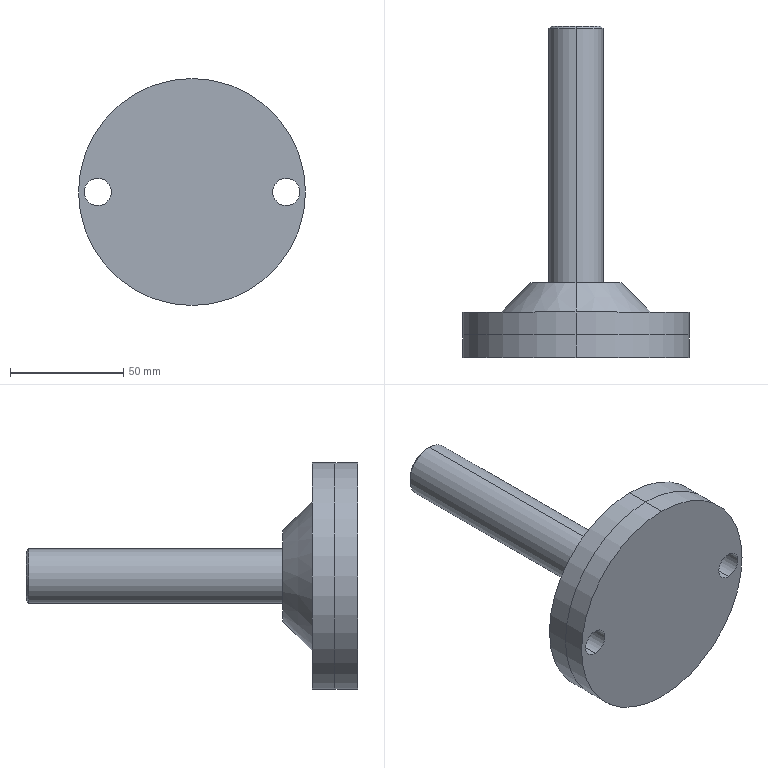Part | SolidWorks | features BaseBody 3 | 3 solids | 41 faces | box 100 x 146 x 100 mm | volume 232661 mm3 | cylinder 18 | plane 15 | cone 8 | commonest cylinder face diameters 12 x8 100 x4 24 x2 26 x2 30 x2
STEP:
#1=CARTESIAN_POINT('',(-41.5,-15.,-6.));
#2=VERTEX_POINT('',#1);
#3=CARTESIAN_POINT('',(-41.5,-15.,6.));
#4=VERTEX_POINT('',#3);
#5=CARTESIAN_POINT('',(-41.5,-15.,0.));
#6=DIRECTION('',(0.,1.,0.));
#7=DIRECTION('',(0.,0.,1.));
#8=AXIS2_PLACEMENT_3D('',#5,#6,#7);
#9=CIRCLE('',#8,6.);
#10=EDGE_CURVE('',#2,#4,#9,.T.);
#11=ORIENTED_EDGE('',*,*,#10,.F.);
#12=CARTESIAN_POINT('',(-41.5,-5.,-6.));
#13=VERTEX_POINT('',#12);
#14=CARTESIAN_POINT('',(-41.5,-15.,-6.));
#15=DIRECTION('',(0.,1.,0.));
#16=VECTOR('',#15,1000.);
#17=LINE('',#14,#16);
#18=EDGE_CURVE('',#2,#13,#17,.T.);
#19=ORIENTED_EDGE('',*,*,#18,.T.);
#20=CARTESIAN_POINT('',(-41.5,-5.,6.));
#21=VERTEX_POINT('',#20);
#22=CARTESIAN_POINT('',(-41.5,-5.,0.));
#23=DIRECTION('',(0.,1.,0.));
#24=DIRECTION('',(0.,0.,1.));
#25=AXIS2_PLACEMENT_3D('',#22,#23,#24);
#26=CIRCLE('',#25,6.);
#27=EDGE_CURVE('',#13,#21,#26,.T.);
#28=ORIENTED_EDGE('',*,*,#27,.T.);
#29=CARTESIAN_POINT('',(-41.5,-15.,6.));
#30=DIRECTION('',(0.,1.,0.));
#31=VECTOR('',#30,1000.);
#32=LINE('',#29,#31);
#33=EDGE_CURVE('',#4,#21,#32,.T.);
#34=ORIENTED_EDGE('',*,*,#33,.F.);
#35=EDGE_LOOP('',(#11,#19,#28,#34));
#36=FACE_OUTER_BOUND('',#35,.T.);
#37=CARTESIAN_POINT('',(-41.5,-15.,0.));
#38=DIRECTION('',(0.,1.,0.));
#39=DIRECTION('',(0.,0.,1.));
#40=AXIS2_PLACEMENT_3D('',#37,#38,#39);
#41=CYLINDRICAL_SURFACE('',#40,6.);
#42=ADVANCED_FACE('',(#36),#41,.F.);
#43=CARTESIAN_POINT('',(41.5,-15.,-6.));
#44=VERTEX_POINT('',#43);
#45=CARTESIAN_POINT('',(41.5,-15.,6.));
#46=VERTEX_POINT('',#45);
#47=CARTESIAN_POINT('',(41.5,-15.,0.));
#48=DIRECTION('',(0.,1.,0.));
#49=DIRECTION('',(0.,0.,1.));
#50=AXIS2_PLACEMENT_3D('',#47,#48,#49);
#51=CIRCLE('',#50,6.);
#52=EDGE_CURVE('',#44,#46,#51,.T.);
#53=ORIENTED_EDGE('',*,*,#52,.F.);
#54=CARTESIAN_POINT('',(41.5,-5.,-6.));
#55=VERTEX_POINT('',#54);
#56=CARTESIAN_POINT('',(41.5,-15.,-6.));
#57=DIRECTION('',(0.,1.,0.));
#58=VECTOR('',#57,1000.);
#59=LINE('',#56,#58);
#60=EDGE_CURVE('',#44,#55,#59,.T.);
#61=ORIENTED_EDGE('',*,*,#60,.T.);
#62=CARTESIAN_POINT('',(41.5,-5.,6.));
#63=VERTEX_POINT('',#62);
#64=CARTESIAN_POINT('',(41.5,-5.,0.));
#65=DIRECTION('',(0.,1.,0.));
#66=DIRECTION('',(0.,0.,1.));
#67=AXIS2_PLACEMENT_3D('',#64,#65,#66);
#68=CIRCLE('',#67,6.);
#69=EDGE_CURVE('',#55,#63,#68,.T.);
#70=ORIENTED_EDGE('',*,*,#69,.T.);
#71=CARTESIAN_POINT('',(41.5,-15.,6.));
#72=DIRECTION('',(0.,1.,0.));
#73=VECTOR('',#72,1000.);
#74=LINE('',#71,#73);
#75=EDGE_CURVE('',#46,#63,#74,.T.);
#76=ORIENTED_EDGE('',*,*,#75,.F.);
#77=EDGE_LOOP('',(#53,#61,#70,#76));
#78=FACE_OUTER_BOUND('',#77,.T.);
#79=CARTESIAN_POINT('',(41.5,-15.,0.));
#80=DIRECTION('',(0.,1.,0.));
#81=DIRECTION('',(0.,0.,1.));
#82=AXIS2_PLACEMENT_3D('',#79,#80,#81);
#83=CYLINDRICAL_SURFACE('',#82,6.);
#84=ADVANCED_FACE('',(#78),#83,.F.);
#85=CARTESIAN_POINT('',(0.,0.,13.));
#86=VERTEX_POINT('',#85);
#87=CARTESIAN_POINT('',(0.,0.,-13.));
#88=VERTEX_POINT('',#87);
#89=CARTESIAN_POINT('',(0.,0.,0.));
#90=DIRECTION('',(0.,-1.,0.));
#91=DIRECTION('',(0.,0.,-1.));
#92=AXIS2_PLACEMENT_3D('',#89,#90,#91);
#93=CIRCLE('',#92,13.);
#94=EDGE_CURVE('',#86,#88,#93,.T.);
#95=ORIENTED_EDGE('',*,*,#94,.T.);
#96=CARTESIAN_POINT('',(0.,8.,-13.));
#97=VERTEX_POINT('',#96);
#98=CARTESIAN_POINT('',(0.,8.,-13.));
#99=DIRECTION('',(0.,1.,0.));
#100=VECTOR('',#99,1000.);
#101=LINE('',#98,#100);
#102=EDGE_CURVE('',#88,#97,#101,.T.);
#103=ORIENTED_EDGE('',*,*,#102,.T.);
#104=CARTESIAN_POINT('',(0.,8.,13.));
#105=VERTEX_POINT('',#104);
#106=CARTESIAN_POINT('',(0.,8.,0.));
#107=DIRECTION('',(0.,1.,0.));
#108=DIRECTION('',(0.,0.,1.));
#109=AXIS2_PLACEMENT_3D('',#106,#107,#108);
#110=CIRCLE('',#109,13.);
#111=EDGE_CURVE('',#97,#105,#110,.T.);
#112=ORIENTED_EDGE('',*,*,#111,.T.);
#113=CARTESIAN_POINT('',(0.,8.,13.));
#114=DIRECTION('',(0.,1.,0.));
#115=VECTOR('',#114,1000.);
#116=LINE('',#113,#115);
#117=EDGE_CURVE('',#86,#105,#116,.T.);
#118=ORIENTED_EDGE('',*,*,#117,.F.);
#119=EDGE_LOOP('',(#95,#103,#112,#118));
#120=FACE_OUTER_BOUND('',#119,.T.);
#121=CARTESIAN_POINT('',(0.,8.,0.));
#122=DIRECTION('',(0.,1.,0.));
#123=DIRECTION('',(0.,0.,1.));
#124=AXIS2_PLACEMENT_3D('',#121,#122,#123);
#125=CYLINDRICAL_SURFACE('',#124,13.);
#126=ADVANCED_FACE('',(#120),#125,.F.);
#127=CARTESIAN_POINT('',(0.,8.,-20.));
#128=VERTEX_POINT('',#127);
#129=CARTESIAN_POINT('',(0.,8.,20.));
#130=VERTEX_POINT('',#129);
#131=CARTESIAN_POINT('',(0.,8.,0.));
#132=DIRECTION('',(0.,-1.,0.));
#133=DIRECTION('',(0.,0.,-1.));
#134=AXIS2_PLACEMENT_3D('',#131,#132,#133);
#135=CIRCLE('',#134,20.);
#136=EDGE_CURVE('',#128,#130,#135,.T.);
#137=ORIENTED_EDGE('',*,*,#136,.T.);
#138=CARTESIAN_POINT('',(0.,-5.,33.));
#139=VERTEX_POINT('',#138);
#140=CARTESIAN_POINT('',(0.,-5.,33.));
#141=DIRECTION('',(0.,-0.7071,0.7071));
#142=VECTOR('',#141,1000.);
#143=LINE('',#140,#142);
#144=EDGE_CURVE('',#130,#139,#143,.T.);
#145=ORIENTED_EDGE('',*,*,#144,.T.);
#146=CARTESIAN_POINT('',(0.,-5.,-33.));
#147=VERTEX_POINT('',#146);
#148=CARTESIAN_POINT('',(0.,-5.,0.));
#149=DIRECTION('',(0.,-1.,0.));
#150=DIRECTION('',(0.,0.,-1.));
#151=AXIS2_PLACEMENT_3D('',#148,#149,#150);
#152=CIRCLE('',#151,33.);
#153=EDGE_CURVE('',#147,#139,#152,.T.);
#154=ORIENTED_EDGE('',*,*,#153,.F.);
#155=CARTESIAN_POINT('',(0.,-5.,-33.));
#156=DIRECTION('',(0.,-0.7071,-0.7071));
#157=VECTOR('',#156,1000.);
#158=LINE('',#155,#157);
#159=EDGE_CURVE('',#128,#147,#158,.T.);
#160=ORIENTED_EDGE('',*,*,#159,.F.);
#161=EDGE_LOOP('',(#137,#145,#154,#160));
#162=FACE_OUTER_BOUND('',#161,.T.);
#163=CARTESIAN_POINT('',(0.,-5.,0.));
#164=DIRECTION('',(0.,-1.,0.));
#165=DIRECTION('',(0.,0.,-1.));
#166=AXIS2_PLACEMENT_3D('',#163,#164,#165);
#167=CONICAL_SURFACE('',#166,33.,0.7854);
#168=ADVANCED_FACE('',(#162),#167,.T.);
#169=CARTESIAN_POINT('',(0.,-5.,-50.));
#170=VERTEX_POINT('',#169);
#171=CARTESIAN_POINT('',(0.,-5.,50.));
#172=VERTEX_POINT('',#171);
#173=CARTESIAN_POINT('',(0.,-5.,0.));
#174=DIRECTION('',(0.,-1.,0.));
#175=DIRECTION('',(0.,0.,-1.));
#176=AXIS2_PLACEMENT_3D('',#173,#174,#175);
#177=CIRCLE('',#176,50.);
#178=EDGE_CURVE('',#170,#172,#177,.T.);
#179=ORIENTED_EDGE('',*,*,#178,.T.);
#180=CARTESIAN_POINT('',(0.,-15.,50.));
#181=VERTEX_POINT('',#180);
#182=CARTESIAN_POINT('',(0.,0.,50.));
#183=DIRECTION('',(0.,-1.,0.));
#184=VECTOR('',#183,1000.);
#185=LINE('',#182,#184);
#186=EDGE_CURVE('',#172,#181,#185,.T.);
#187=ORIENTED_EDGE('',*,*,#186,.T.);
#188=CARTESIAN_POINT('',(0.,-15.,-50.));
#189=VERTEX_POINT('',#188);
#190=CARTESIAN_POINT('',(0.,-15.,0.));
#191=DIRECTION('',(0.,-1.,0.));
#192=DIRECTION('',(0.,0.,-1.));
#193=AXIS2_PLACEMENT_3D('',#190,#191,#192);
#194=CIRCLE('',#193,50.);
#195=EDGE_CURVE('',#189,#181,#194,.T.);
#196=ORIENTED_EDGE('',*,*,#195,.F.);
#197=CARTESIAN_POINT('',(0.,0.,-50.));
#198=DIRECTION('',(0.,-1.,0.));
#199=VECTOR('',#198,1000.);
#200=LINE('',#197,#199);
#201=EDGE_CURVE('',#170,#189,#200,.T.);
#202=ORIENTED_EDGE('',*,*,#201,.F.);
#203=EDGE_LOOP('',(#179,#187,#196,#202));
#204=FACE_OUTER_BOUND('',#203,.T.);
#205=CARTESIAN_POINT('',(0.,0.,0.));
#206=DIRECTION('',(0.,-1.,0.));
#207=DIRECTION('',(0.,0.,-1.));
#208=AXIS2_PLACEMENT_3D('',#205,#206,#207);
#209=CYLINDRICAL_SURFACE('',#208,50.);
#210=ADVANCED_FACE('',(#204),#209,.T.);
#211=CARTESIAN_POINT('',(0.,0.,15.));
#212=VERTEX_POINT('',#211);
#213=CARTESIAN_POINT('',(0.,0.,-15.));
#214=VERTEX_POINT('',#213);
#215=CARTESIAN_POINT('',(0.,0.,0.));
#216=DIRECTION('',(0.,-1.,0.));
#217=DIRECTION('',(0.,0.,-1.));
#218=AXIS2_PLACEMENT_3D('',#215,#216,#217);
#219=CIRCLE('',#218,15.);
#220=EDGE_CURVE('',#212,#214,#219,.T.);
#221=ORIENTED_EDGE('',*,*,#220,.F.);
#222=CARTESIAN_POINT('',(0.,-15.,15.));
#223=VERTEX_POINT('',#222);
#224=CARTESIAN_POINT('',(0.,0.,15.));
#225=DIRECTION('',(0.,-1.,0.));
#226=VECTOR('',#225,1000.);
#227=LINE('',#224,#226);
#228=EDGE_CURVE('',#212,#223,#227,.T.);
#229=ORIENTED_EDGE('',*,*,#228,.T.);
#230=CARTESIAN_POINT('',(0.,-15.,-15.));
#231=VERTEX_POINT('',#230);
#232=CARTESIAN_POINT('',(0.,-15.,0.));
#233=DIRECTION('',(0.,-1.,0.));
#234=DIRECTION('',(0.,0.,-1.));
#235=AXIS2_PLACEMENT_3D('',#232,#233,#234);
#236=CIRCLE('',#235,15.);
#237=EDGE_CURVE('',#223,#231,#236,.T.);
#238=ORIENTED_EDGE('',*,*,#237,.T.);
#239=CARTESIAN_POINT('',(0.,0.,-15.));
#240=DIRECTION('',(0.,-1.,0.));
#241=VECTOR('',#240,1000.);
#242=LINE('',#239,#241);
#243=EDGE_CURVE('',#214,#231,#242,.T.);
#244=ORIENTED_EDGE('',*,*,#243,.F.);
#245=EDGE_LOOP('',(#221,#229,#238,#244));
#246=FACE_OUTER_BOUND('',#245,.T.);
#247=CARTESIAN_POINT('',(0.,0.,0.));
#248=DIRECTION('',(0.,-1.,0.));
#249=DIRECTION('',(0.,0.,-1.));
#250=AXIS2_PLACEMENT_3D('',#247,#248,#249);
#251=CYLINDRICAL_SURFACE('',#250,15.);
#252=ADVANCED_FACE('',(#246),#251,.F.);
#253=ORIENTED_EDGE('',*,*,#94,.F.);
#254=CARTESIAN_POINT('',(0.,0.,0.));
#255=DIRECTION('',(0.,-1.,0.));
#256=DIRECTION('',(0.,0.,-1.));
#257=AXIS2_PLACEMENT_3D('',#254,#255,#256);
#258=CIRCLE('',#257,13.);
#259=EDGE_CURVE('',#88,#86,#258,.T.);
#260=ORIENTED_EDGE('',*,*,#259,.F.);
#261=EDGE_LOOP('',(#253,#260));
#262=FACE_BOUND('',#261,.T.);
#263=CARTESIAN_POINT('',(0.,0.,0.));
#264=DIRECTION('',(0.,-1.,0.));
#265=DIRECTION('',(0.,0.,-1.));
#266=AXIS2_PLACEMENT_3D('',#263,#264,#265);
#267=CIRCLE('',#266,15.);
#268=EDGE_CURVE('',#214,#212,#267,.T.);
#269=ORIENTED_EDGE('',*,*,#268,.T.);
#270=ORIENTED_EDGE('',*,*,#220,.T.);
#271=EDGE_LOOP('',(#269,#270));
#272=FACE_OUTER_BOUND('',#271,.T.);
#273=CARTESIAN_POINT('',(0.,0.,0.));
#274=DIRECTION('',(0.,-1.,0.));
#275=DIRECTION('',(0.,0.,-1.));
#276=AXIS2_PLACEMENT_3D('',#273,#274,#275);
#277=PLANE('',#276);
#278=ADVANCED_FACE('',(#262,#272),#277,.T.);
#279=ORIENTED_EDGE('',*,*,#228,.F.);
#280=ORIENTED_EDGE('',*,*,#268,.F.);
#281=ORIENTED_EDGE('',*,*,#243,.T.);
#282=CARTESIAN_POINT('',(0.,-15.,0.));
#283=DIRECTION('',(0.,-1.,0.));
#284=DIRECTION('',(0.,0.,-1.));
#285=AXIS2_PLACEMENT_3D('',#282,#283,#284);
#286=CIRCLE('',#285,15.);
#287=EDGE_CURVE('',#231,#223,#286,.T.);
#288=ORIENTED_EDGE('',*,*,#287,.T.);
#289=EDGE_LOOP('',(#279,#280,#281,#288));
#290=FACE_OUTER_BOUND('',#289,.T.);
#291=CARTESIAN_POINT('',(0.,0.,0.));
#292=DIRECTION('',(0.,-1.,0.));
#293=DIRECTION('',(0.,0.,-1.));
#294=AXIS2_PLACEMENT_3D('',#291,#292,#293);
#295=CYLINDRICAL_SURFACE('',#294,15.);
#296=ADVANCED_FACE('',(#290),#295,.F.);
#297=CARTESIAN_POINT('',(-41.5,-15.,0.));
#298=DIRECTION('',(0.,1.,0.));
#299=DIRECTION('',(0.,0.,1.));
#300=AXIS2_PLACEMENT_3D('',#297,#298,#299);
#301=CIRCLE('',#300,6.);
#302=EDGE_CURVE('',#4,#2,#301,.T.);
#303=ORIENTED_EDGE('',*,*,#302,.T.);
#304=ORIENTED_EDGE('',*,*,#10,.T.);
#305=EDGE_LOOP('',(#303,#304));
#306=FACE_BOUND('',#305,.T.);
#307=CARTESIAN_POINT('',(41.5,-15.,0.));
#308=DIRECTION('',(0.,1.,0.));
#309=DIRECTION('',(0.,0.,1.));
#310=AXIS2_PLACEMENT_3D('',#307,#308,#309);
#311=CIRCLE('',#310,6.);
#312=EDGE_CURVE('',#46,#44,#311,.T.);
#313=ORIENTED_EDGE('',*,*,#312,.T.);
#314=ORIENTED_EDGE('',*,*,#52,.T.);
#315=EDGE_LOOP('',(#313,#314));
#316=FACE_BOUND('',#315,.T.);
#317=ORIENTED_EDGE('',*,*,#195,.T.);
#318=CARTESIAN_POINT('',(0.,-15.,0.));
#319=DIRECTION('',(0.,-1.,0.));
#320=DIRECTION('',(0.,0.,-1.));
#321=AXIS2_PLACEMENT_3D('',#318,#319,#320);
#322=CIRCLE('',#321,50.);
#323=EDGE_CURVE('',#181,#189,#322,.T.);
#324=ORIENTED_EDGE('',*,*,#323,.T.);
#325=EDGE_LOOP('',(#317,#324));
#326=FACE_OUTER_BOUND('',#325,.T.);
#327=ORIENTED_EDGE('',*,*,#287,.F.);
#328=ORIENTED_EDGE('',*,*,#237,.F.);
#329=EDGE_LOOP('',(#327,#328));
#330=FACE_BOUND('',#329,.T.);
#331=CARTESIAN_POINT('',(15.,-15.,0.));
#332=DIRECTION('',(0.,-1.,0.));
#333=DIRECTION('',(0.,0.,-1.));
#334=AXIS2_PLACEMENT_3D('',#331,#332,#333);
#335=PLANE('',#334);
#336=ADVANCED_FACE('',(#306,#316,#326,#330),#335,.T.);
#337=ORIENTED_EDGE('',*,*,#186,.F.);
#338=CARTESIAN_POINT('',(0.,-5.,0.));
#339=DIRECTION('',(0.,-1.,0.));
#340=DIRECTION('',(0.,0.,-1.));
#341=AXIS2_PLACEMENT_3D('',#338,#339,#340);
#342=CIRCLE('',#341,50.);
#343=EDGE_CURVE('',#172,#170,#342,.T.);
#344=ORIENTED_EDGE('',*,*,#343,.T.);
#345=ORIENTED_EDGE('',*,*,#201,.T.);
#346=ORIENTED_EDGE('',*,*,#323,.F.);
#347=EDGE_LOOP('',(#337,#344,#345,#346));
#348=FACE_OUTER_BOUND('',#347,.T.);
#349=CARTESIAN_POINT('',(0.,0.,0.));
#350=DIRECTION('',(0.,-1.,0.));
#351=DIRECTION('',(0.,0.,-1.));
#352=AXIS2_PLACEMENT_3D('',#349,#350,#351);
#353=CYLINDRICAL_SURFACE('',#352,50.);
#354=ADVANCED_FACE('',(#348),#353,.T.);
#355=CARTESIAN_POINT('',(-41.5,-5.,0.));
#356=DIRECTION('',(0.,1.,0.));
#357=DIRECTION('',(0.,0.,1.));
#358=AXIS2_PLACEMENT_3D('',#355,#356,#357);
#359=CIRCLE('',#358,6.);
#360=EDGE_CURVE('',#21,#13,#359,.T.);
#361=ORIENTED_EDGE('',*,*,#360,.F.);
#362=ORIENTED_EDGE('',*,*,#27,.F.);
#363=EDGE_LOOP('',(#361,#362));
#364=FACE_BOUND('',#363,.T.);
#365=CARTESIAN_POINT('',(41.5,-5.,0.));
#366=DIRECTION('',(0.,1.,0.));
#367=DIRECTION('',(0.,0.,1.));
#368=AXIS2_PLACEMENT_3D('',#365,#366,#367);
#369=CIRCLE('',#368,6.);
#370=EDGE_CURVE('',#63,#55,#369,.T.);
#371=ORIENTED_EDGE('',*,*,#370,.F.);
#372=ORIENTED_EDGE('',*,*,#69,.F.);
#373=EDGE_LOOP('',(#371,#372));
#374=FACE_BOUND('',#373,.T.);
#375=ORIENTED_EDGE('',*,*,#153,.T.);
#376=CARTESIAN_POINT('',(0.,-5.,0.));
#377=DIRECTION('',(0.,-1.,0.));
#378=DIRECTION('',(0.,0.,-1.));
#379=AXIS2_PLACEMENT_3D('',#376,#377,#378);
#380=CIRCLE('',#379,33.);
#381=EDGE_CURVE('',#139,#147,#380,.T.);
#382=ORIENTED_EDGE('',*,*,#381,.T.);
#383=EDGE_LOOP('',(#375,#382));
#384=FACE_BOUND('',#383,.T.);
#385=ORIENTED_EDGE('',*,*,#178,.F.);
#386=ORIENTED_EDGE('',*,*,#343,.F.);
#387=EDGE_LOOP('',(#385,#386));
#388=FACE_OUTER_BOUND('',#387,.T.);
#389=CARTESIAN_POINT('',(50.,-5.,0.));
#390=DIRECTION('',(0.,1.,0.));
#391=DIRECTION('',(0.,0.,1.));
#392=AXIS2_PLACEMENT_3D('',#389,#390,#391);
#393=PLANE('',#392);
#394=ADVANCED_FACE('',(#364,#374,#384,#388),#393,.T.);
#395=ORIENTED_EDGE('',*,*,#144,.F.);
#396=CARTESIAN_POINT('',(0.,8.,0.));
#397=DIRECTION('',(0.,-1.,0.));
#398=DIRECTION('',(0.,0.,-1.));
#399=AXIS2_PLACEMENT_3D('',#396,#397,#398);
#400=CIRCLE('',#399,20.);
#401=EDGE_CURVE('',#130,#128,#400,.T.);
#402=ORIENTED_EDGE('',*,*,#401,.T.);
#403=ORIENTED_EDGE('',*,*,#159,.T.);
#404=ORIENTED_EDGE('',*,*,#381,.F.);
#405=EDGE_LOOP('',(#395,#402,#403,#404));
#406=FACE_OUTER_BOUND('',#405,.T.);
#407=CARTESIAN_POINT('',(0.,-5.,0.));
#408=DIRECTION('',(0.,-1.,0.));
#409=DIRECTION('',(0.,0.,-1.));
#410=AXIS2_PLACEMENT_3D('',#407,#408,#409);
#411=CONICAL_SURFACE('',#410,33.,0.7854);
#412=ADVANCED_FACE('',(#406),#411,.T.);
#413=CARTESIAN_POINT('',(0.,8.,0.));
#414=DIRECTION('',(0.,1.,0.));
#415=DIRECTION('',(0.,0.,1.));
#416=AXIS2_PLACEMENT_3D('',#413,#414,#415);
#417=CIRCLE('',#416,13.);
#418=EDGE_CURVE('',#105,#97,#417,.T.);
#419=ORIENTED_EDGE('',*,*,#418,.F.);
#420=ORIENTED_EDGE('',*,*,#111,.F.);
#421=EDGE_LOOP('',(#419,#420));
#422=FACE_BOUND('',#421,.T.);
#423=ORIENTED_EDGE('',*,*,#136,.F.);
#424=ORIENTED_EDGE('',*,*,#401,.F.);
#425=EDGE_LOOP('',(#423,#424));
#426=FACE_OUTER_BOUND('',#425,.T.);
#427=CARTESIAN_POINT('',(20.,8.,0.));
#428=DIRECTION('',(0.,1.,0.));
#429=DIRECTION('',(0.,0.,1.));
#430=AXIS2_PLACEMENT_3D('',#427,#428,#429);
#431=PLANE('',#430);
#432=ADVANCED_FACE('',(#422,#426),#431,.T.);
#433=ORIENTED_EDGE('',*,*,#102,.F.);
#434=ORIENTED_EDGE('',*,*,#259,.T.);
#435=ORIENTED_EDGE('',*,*,#117,.T.);
#436=ORIENTED_EDGE('',*,*,#418,.T.);
#437=EDGE_LOOP('',(#433,#434,#435,#436));
#438=FACE_OUTER_BOUND('',#437,.T.);
#439=CARTESIAN_POINT('',(0.,8.,0.));
#440=DIRECTION('',(0.,1.,0.));
#441=DIRECTION('',(0.,0.,1.));
#442=AXIS2_PLACEMENT_3D('',#439,#440,#441);
#443=CYLINDRICAL_SURFACE('',#442,13.);
#444=ADVANCED_FACE('',(#438),#443,.F.);
#445=ORIENTED_EDGE('',*,*,#60,.F.);
#446=ORIENTED_EDGE('',*,*,#312,.F.);
#447=ORIENTED_EDGE('',*,*,#75,.T.);
#448=ORIENTED_EDGE('',*,*,#370,.T.);
#449=EDGE_LOOP('',(#445,#446,#447,#448));
#450=FACE_OUTER_BOUND('',#449,.T.);
#451=CARTESIAN_POINT('',(41.5,-15.,0.));
#452=DIRECTION('',(0.,1.,0.));
#453=DIRECTION('',(0.,0.,1.));
#454=AXIS2_PLACEMENT_3D('',#451,#452,#453);
#455=CYLINDRICAL_SURFACE('',#454,6.);
#456=ADVANCED_FACE('',(#450),#455,.F.);
#457=ORIENTED_EDGE('',*,*,#18,.F.);
#458=ORIENTED_EDGE('',*,*,#302,.F.);
#459=ORIENTED_EDGE('',*,*,#33,.T.);
#460=ORIENTED_EDGE('',*,*,#360,.T.);
#461=EDGE_LOOP('',(#457,#458,#459,#460));
#462=FACE_OUTER_BOUND('',#461,.T.);
#463=CARTESIAN_POINT('',(-41.5,-15.,0.));
#464=DIRECTION('',(0.,1.,0.));
#465=DIRECTION('',(0.,0.,1.));
#466=AXIS2_PLACEMENT_3D('',#463,#464,#465);
#467=CYLINDRICAL_SURFACE('',#466,6.);
#468=ADVANCED_FACE('',(#462),#467,.F.);
#469=CLOSED_SHELL('',(#42,#84,#126,#168,#210,#252,#278,#296,#336,#354,#394,#412,#432,#444,#456,#468));
#470=MANIFOLD_SOLID_BREP('',#469);
#471=CARTESIAN_POINT('',(0.,121.,11.));
#472=VERTEX_POINT('',#471);
#473=CARTESIAN_POINT('',(0.,121.,-11.));
#474=VERTEX_POINT('',#473);
#475=CARTESIAN_POINT('',(0.,121.,0.));
#476=DIRECTION('',(0.,1.,0.));
#477=DIRECTION('',(0.,0.,-1.));
#478=AXIS2_PLACEMENT_3D('',#475,#476,#477);
#479=CIRCLE('',#478,11.);
#480=EDGE_CURVE('',#472,#474,#479,.T.);
#481=ORIENTED_EDGE('',*,*,#480,.F.);
#482=CARTESIAN_POINT('',(0.,120.,12.));
#483=VERTEX_POINT('',#482);
#484=CARTESIAN_POINT('',(0.,120.,12.));
#485=DIRECTION('',(0.,-0.7071,0.7071));
#486=VECTOR('',#485,1000.);
#487=LINE('',#484,#486);
#488=EDGE_CURVE('',#472,#483,#487,.T.);
#489=ORIENTED_EDGE('',*,*,#488,.T.);
#490=CARTESIAN_POINT('',(0.,120.,-12.));
#491=VERTEX_POINT('',#490);
#492=CARTESIAN_POINT('',(0.,120.,0.));
#493=DIRECTION('',(0.,-1.,0.));
#494=DIRECTION('',(0.,0.,-1.));
#495=AXIS2_PLACEMENT_3D('',#492,#493,#494);
#496=CIRCLE('',#495,12.);
#497=EDGE_CURVE('',#491,#483,#496,.T.);
#498=ORIENTED_EDGE('',*,*,#497,.F.);
#499=CARTESIAN_POINT('',(0.,120.,-12.));
#500=DIRECTION('',(0.,-0.7071,-0.7071));
#501=VECTOR('',#500,1000.);
#502=LINE('',#499,#501);
#503=EDGE_CURVE('',#474,#491,#502,.T.);
#504=ORIENTED_EDGE('',*,*,#503,.F.);
#505=EDGE_LOOP('',(#481,#489,#498,#504));
#506=FACE_OUTER_BOUND('',#505,.T.);
#507=CARTESIAN_POINT('',(0.,120.,0.));
#508=DIRECTION('',(0.,-1.,0.));
#509=DIRECTION('',(0.,0.,-1.));
#510=AXIS2_PLACEMENT_3D('',#507,#508,#509);
#511=CONICAL_SURFACE('',#510,12.,0.7854);
#512=ADVANCED_FACE('',(#506),#511,.T.);
#513=ORIENTED_EDGE('',*,*,#497,.T.);
#514=CARTESIAN_POINT('',(0.,0.,12.));
#515=VERTEX_POINT('',#514);
#516=CARTESIAN_POINT('',(0.,121.,12.));
#517=DIRECTION('',(0.,-1.,0.));
#518=VECTOR('',#517,1000.);
#519=LINE('',#516,#518);
#520=EDGE_CURVE('',#483,#515,#519,.T.);
#521=ORIENTED_EDGE('',*,*,#520,.T.);
#522=CARTESIAN_POINT('',(0.,0.,-12.));
#523=VERTEX_POINT('',#522);
#524=CARTESIAN_POINT('',(0.,0.,0.));
#525=DIRECTION('',(0.,1.,0.));
#526=DIRECTION('',(0.,0.,-1.));
#527=AXIS2_PLACEMENT_3D('',#524,#525,#526);
#528=CIRCLE('',#527,12.);
#529=EDGE_CURVE('',#515,#523,#528,.T.);
#530=ORIENTED_EDGE('',*,*,#529,.T.);
#531=CARTESIAN_POINT('',(0.,121.,-12.));
#532=DIRECTION('',(0.,-1.,0.));
#533=VECTOR('',#532,1000.);
#534=LINE('',#531,#533);
#535=EDGE_CURVE('',#491,#523,#534,.T.);
#536=ORIENTED_EDGE('',*,*,#535,.F.);
#537=EDGE_LOOP('',(#513,#521,#530,#536));
#538=FACE_OUTER_BOUND('',#537,.T.);
#539=CARTESIAN_POINT('',(0.,121.,0.));
#540=DIRECTION('',(0.,-1.,0.));
#541=DIRECTION('',(0.,0.,-1.));
#542=AXIS2_PLACEMENT_3D('',#539,#540,#541);
#543=CYLINDRICAL_SURFACE('',#542,12.);
#544=ADVANCED_FACE('',(#538),#543,.T.);
#545=CARTESIAN_POINT('',(0.,0.,17.785));
#546=VERTEX_POINT('',#545);
#547=CARTESIAN_POINT('',(0.,0.,-17.785));
#548=VERTEX_POINT('',#547);
#549=CARTESIAN_POINT('',(0.,0.,0.));
#550=DIRECTION('',(0.,1.,0.));
#551=DIRECTION('',(0.,0.,-1.));
#552=AXIS2_PLACEMENT_3D('',#549,#550,#551);
#553=CIRCLE('',#552,17.785);
#554=EDGE_CURVE('',#546,#548,#553,.T.);
#555=ORIENTED_EDGE('',*,*,#554,.F.);
#556=CARTESIAN_POINT('',(0.,-0.2154,18.));
#557=VERTEX_POINT('',#556);
#558=CARTESIAN_POINT('',(0.,-3.,20.785));
#559=DIRECTION('',(0.,-0.7071,0.7071));
#560=VECTOR('',#559,1000.);
#561=LINE('',#558,#560);
#562=EDGE_CURVE('',#546,#557,#561,.T.);
#563=ORIENTED_EDGE('',*,*,#562,.T.);
#564=CARTESIAN_POINT('',(10.392,-3.,18.));
#565=VERTEX_POINT('',#564);
#566=CARTESIAN_POINT('',(0.,-0.2154,18.));
#567=CARTESIAN_POINT('',(0.4549,-0.2154,18.));
#568=CARTESIAN_POINT('',(0.9142,-0.2329,18.));
#569=CARTESIAN_POINT('',(1.821,-0.3016,18.));
#570=CARTESIAN_POINT('',(2.271,-0.3527,18.));
#571=CARTESIAN_POINT('',(3.609,-0.5525,18.));
#572=CARTESIAN_POINT('',(4.487,-0.7477,18.));
#573=CARTESIAN_POINT('',(6.219,-1.241,18.));
#574=CARTESIAN_POINT('',(7.073,-1.54,18.));
#575=CARTESIAN_POINT('',(8.762,-2.22,18.));
#576=CARTESIAN_POINT('',(9.586,-2.597,18.));
#577=CARTESIAN_POINT('',(10.392,-3.,18.));
#578=B_SPLINE_CURVE_WITH_KNOTS('',3,(#566,#567,#568,#569,#570,#571,#572,#573,#574,#575,#576,#577),.UNSPECIFIED.,.F.,.F.,(4,2,2,2,2,4),(0.03698,0.03833,0.03968,0.04238,0.04509,0.04779),.UNSPECIFIED.);
#579=EDGE_CURVE('',#557,#565,#578,.T.);
#580=ORIENTED_EDGE('',*,*,#579,.T.);
#581=CARTESIAN_POINT('',(20.785,-3.,0.));
#582=VERTEX_POINT('',#581);
#583=CARTESIAN_POINT('',(10.392,-3.,18.));
#584=CARTESIAN_POINT('',(11.204,-2.188,16.594));
#585=CARTESIAN_POINT('',(12.035,-1.498,15.156));
#586=CARTESIAN_POINT('',(13.325,-0.7578,12.921));
#587=CARTESIAN_POINT('',(13.762,-0.561,12.163));
#588=CARTESIAN_POINT('',(14.432,-0.358,11.003));
#589=CARTESIAN_POINT('',(14.658,-0.3056,10.612));
#590=CARTESIAN_POINT('',(15.114,-0.2346,9.821));
#591=CARTESIAN_POINT('',(15.343,-0.2164,9.426));
#592=CARTESIAN_POINT('',(16.477,-0.2116,7.462));
#593=CARTESIAN_POINT('',(17.368,-0.4863,5.917));
#594=CARTESIAN_POINT('',(19.127,-1.483,2.871));
#595=CARTESIAN_POINT('',(19.968,-2.183,1.415));
#596=CARTESIAN_POINT('',(20.785,-3.,0.));
#597=B_SPLINE_CURVE_WITH_KNOTS('',3,(#583,#584,#585,#586,#587,#588,#589,#590,#591,#592,#593,#594,#595,#596),.UNSPECIFIED.,.F.,.F.,(4,2,2,2,2,2,4),(0.000000254,0.005368,0.008051,0.009393,0.01074,0.0161,0.02147),.UNSPECIFIED.);
#598=EDGE_CURVE('',#565,#582,#597,.T.);
#599=ORIENTED_EDGE('',*,*,#598,.T.);
#600=CARTESIAN_POINT('',(10.392,-3.,-18.));
#601=VERTEX_POINT('',#600);
#602=CARTESIAN_POINT('',(20.785,-3.,0.));
#603=CARTESIAN_POINT('',(19.973,-2.188,-1.406));
#604=CARTESIAN_POINT('',(19.142,-1.498,-2.844));
#605=CARTESIAN_POINT('',(17.852,-0.7578,-5.079));
#606=CARTESIAN_POINT('',(17.415,-0.561,-5.837));
#607=CARTESIAN_POINT('',(16.745,-0.358,-6.997));
#608=CARTESIAN_POINT('',(16.519,-0.3056,-7.388));
#609=CARTESIAN_POINT('',(16.063,-0.2346,-8.179));
#610=CARTESIAN_POINT('',(15.834,-0.2164,-8.574));
#611=CARTESIAN_POINT('',(14.7,-0.2116,-10.538));
#612=CARTESIAN_POINT('',(13.809,-0.4863,-12.083));
#613=CARTESIAN_POINT('',(12.05,-1.483,-15.129));
#614=CARTESIAN_POINT('',(11.209,-2.183,-16.585));
#615=CARTESIAN_POINT('',(10.392,-3.,-18.));
#616=B_SPLINE_CURVE_WITH_KNOTS('',3,(#602,#603,#604,#605,#606,#607,#608,#609,#610,#611,#612,#613,#614,#615),.UNSPECIFIED.,.F.,.F.,(4,2,2,2,2,2,4),(0.000000254,0.005368,0.008051,0.009393,0.01074,0.0161,0.02147),.UNSPECIFIED.);
#617=EDGE_CURVE('',#582,#601,#616,.T.);
#618=ORIENTED_EDGE('',*,*,#617,.T.);
#619=CARTESIAN_POINT('',(0.,-0.2154,-18.));
#620=VERTEX_POINT('',#619);
#621=CARTESIAN_POINT('',(10.392,-3.,-18.));
#622=CARTESIAN_POINT('',(9.587,-2.597,-18.));
#623=CARTESIAN_POINT('',(8.766,-2.222,-18.));
#624=CARTESIAN_POINT('',(7.082,-1.543,-18.));
#625=CARTESIAN_POINT('',(6.215,-1.24,-18.));
#626=CARTESIAN_POINT('',(3.602,-0.4961,-18.));
#627=CARTESIAN_POINT('',(1.824,-0.2154,-18.));
#628=CARTESIAN_POINT('',(0.,-0.2154,-18.));
#629=B_SPLINE_CURVE_WITH_KNOTS('',3,(#621,#622,#623,#624,#625,#626,#627,#628),.UNSPECIFIED.,.F.,.F.,(4,2,2,4),(0.02614,0.02885,0.03156,0.03698),.UNSPECIFIED.);
#630=EDGE_CURVE('',#601,#620,#629,.T.);
#631=ORIENTED_EDGE('',*,*,#630,.T.);
#632=CARTESIAN_POINT('',(0.,-3.,-20.785));
#633=DIRECTION('',(0.,-0.7071,-0.7071));
#634=VECTOR('',#633,1000.);
#635=LINE('',#632,#634);
#636=EDGE_CURVE('',#548,#620,#635,.T.);
#637=ORIENTED_EDGE('',*,*,#636,.F.);
#638=EDGE_LOOP('',(#555,#563,#580,#599,#618,#631,#637));
#639=FACE_OUTER_BOUND('',#638,.T.);
#640=CARTESIAN_POINT('',(0.,-3.,0.));
#641=DIRECTION('',(0.,-1.,0.));
#642=DIRECTION('',(0.,0.,-1.));
#643=AXIS2_PLACEMENT_3D('',#640,#641,#642);
#644=CONICAL_SURFACE('',#643,20.785,0.7854);
#645=ADVANCED_FACE('',(#639),#644,.T.);
#646=CARTESIAN_POINT('',(0.,-10.,-17.785));
#647=VERTEX_POINT('',#646);
#648=CARTESIAN_POINT('',(0.,-10.,17.785));
#649=VERTEX_POINT('',#648);
#650=CARTESIAN_POINT('',(0.,-10.,0.));
#651=DIRECTION('',(0.,-1.,0.));
#652=DIRECTION('',(0.,0.,-1.));
#653=AXIS2_PLACEMENT_3D('',#650,#651,#652);
#654=CIRCLE('',#653,17.785);
#655=EDGE_CURVE('',#647,#649,#654,.T.);
#656=ORIENTED_EDGE('',*,*,#655,.F.);
#657=CARTESIAN_POINT('',(0.,-9.785,-18.));
#658=VERTEX_POINT('',#657);
#659=CARTESIAN_POINT('',(0.,-10.,-17.785));
#660=DIRECTION('',(0.,0.7071,-0.7071));
#661=VECTOR('',#660,1000.);
#662=LINE('',#659,#661);
#663=EDGE_CURVE('',#647,#658,#662,.T.);
#664=ORIENTED_EDGE('',*,*,#663,.T.);
#665=CARTESIAN_POINT('',(10.392,-7.,-18.));
#666=VERTEX_POINT('',#665);
#667=CARTESIAN_POINT('',(0.,-9.785,-18.));
#668=CARTESIAN_POINT('',(0.4549,-9.785,-18.));
#669=CARTESIAN_POINT('',(0.9142,-9.767,-18.));
#670=CARTESIAN_POINT('',(1.821,-9.698,-18.));
#671=CARTESIAN_POINT('',(2.271,-9.647,-18.));
#672=CARTESIAN_POINT('',(3.609,-9.448,-18.));
#673=CARTESIAN_POINT('',(4.487,-9.252,-18.));
#674=CARTESIAN_POINT('',(6.219,-8.759,-18.));
#675=CARTESIAN_POINT('',(7.073,-8.46,-18.));
#676=CARTESIAN_POINT('',(8.762,-7.78,-18.));
#677=CARTESIAN_POINT('',(9.586,-7.403,-18.));
#678=CARTESIAN_POINT('',(10.392,-7.,-18.));
#679=B_SPLINE_CURVE_WITH_KNOTS('',3,(#667,#668,#669,#670,#671,#672,#673,#674,#675,#676,#677,#678),.UNSPECIFIED.,.F.,.F.,(4,2,2,2,2,4),(0.03698,0.03833,0.03968,0.04238,0.04509,0.04779),.UNSPECIFIED.);
#680=EDGE_CURVE('',#658,#666,#679,.T.);
#681=ORIENTED_EDGE('',*,*,#680,.T.);
#682=CARTESIAN_POINT('',(20.785,-7.,0.));
#683=VERTEX_POINT('',#682);
#684=CARTESIAN_POINT('',(10.392,-7.,-18.));
#685=CARTESIAN_POINT('',(11.204,-7.812,-16.594));
#686=CARTESIAN_POINT('',(12.035,-8.502,-15.156));
#687=CARTESIAN_POINT('',(13.325,-9.242,-12.921));
#688=CARTESIAN_POINT('',(13.762,-9.439,-12.163));
#689=CARTESIAN_POINT('',(14.432,-9.642,-11.003));
#690=CARTESIAN_POINT('',(14.658,-9.694,-10.612));
#691=CARTESIAN_POINT('',(15.114,-9.765,-9.821));
#692=CARTESIAN_POINT('',(15.343,-9.784,-9.426));
#693=CARTESIAN_POINT('',(16.477,-9.788,-7.462));
#694=CARTESIAN_POINT('',(17.368,-9.514,-5.917));
#695=CARTESIAN_POINT('',(19.127,-8.517,-2.871));
#696=CARTESIAN_POINT('',(19.968,-7.817,-1.415));
#697=CARTESIAN_POINT('',(20.785,-7.,0.));
#698=B_SPLINE_CURVE_WITH_KNOTS('',3,(#684,#685,#686,#687,#688,#689,#690,#691,#692,#693,#694,#695,#696,#697),.UNSPECIFIED.,.F.,.F.,(4,2,2,2,2,2,4),(0.000000254,0.005368,0.008051,0.009393,0.01074,0.0161,0.02147),.UNSPECIFIED.);
#699=EDGE_CURVE('',#666,#683,#698,.T.);
#700=ORIENTED_EDGE('',*,*,#699,.T.);
#701=CARTESIAN_POINT('',(10.392,-7.,18.));
#702=VERTEX_POINT('',#701);
#703=CARTESIAN_POINT('',(20.785,-7.,0.));
#704=CARTESIAN_POINT('',(19.973,-7.812,1.406));
#705=CARTESIAN_POINT('',(19.142,-8.502,2.844));
#706=CARTESIAN_POINT('',(17.852,-9.242,5.079));
#707=CARTESIAN_POINT('',(17.415,-9.439,5.837));
#708=CARTESIAN_POINT('',(16.745,-9.642,6.997));
#709=CARTESIAN_POINT('',(16.519,-9.694,7.388));
#710=CARTESIAN_POINT('',(16.063,-9.765,8.179));
#711=CARTESIAN_POINT('',(15.834,-9.784,8.574));
#712=CARTESIAN_POINT('',(14.7,-9.788,10.538));
#713=CARTESIAN_POINT('',(13.809,-9.514,12.083));
#714=CARTESIAN_POINT('',(12.05,-8.517,15.129));
#715=CARTESIAN_POINT('',(11.209,-7.817,16.585));
#716=CARTESIAN_POINT('',(10.392,-7.,18.));
#717=B_SPLINE_CURVE_WITH_KNOTS('',3,(#703,#704,#705,#706,#707,#708,#709,#710,#711,#712,#713,#714,#715,#716),.UNSPECIFIED.,.F.,.F.,(4,2,2,2,2,2,4),(0.000000254,0.005368,0.008051,0.009393,0.01074,0.0161,0.02147),.UNSPECIFIED.);
#718=EDGE_CURVE('',#683,#702,#717,.T.);
#719=ORIENTED_EDGE('',*,*,#718,.T.);
#720=CARTESIAN_POINT('',(0.,-9.785,18.));
#721=VERTEX_POINT('',#720);
#722=CARTESIAN_POINT('',(10.392,-7.,18.));
#723=CARTESIAN_POINT('',(9.587,-7.403,18.));
#724=CARTESIAN_POINT('',(8.766,-7.778,18.));
#725=CARTESIAN_POINT('',(7.082,-8.457,18.));
#726=CARTESIAN_POINT('',(6.215,-8.76,18.));
#727=CARTESIAN_POINT('',(3.602,-9.504,18.));
#728=CARTESIAN_POINT('',(1.824,-9.785,18.));
#729=CARTESIAN_POINT('',(0.,-9.785,18.));
#730=B_SPLINE_CURVE_WITH_KNOTS('',3,(#722,#723,#724,#725,#726,#727,#728,#729),.UNSPECIFIED.,.F.,.F.,(4,2,2,4),(0.02614,0.02885,0.03156,0.03698),.UNSPECIFIED.);
#731=EDGE_CURVE('',#702,#721,#730,.T.);
#732=ORIENTED_EDGE('',*,*,#731,.T.);
#733=CARTESIAN_POINT('',(0.,-10.,17.785));
#734=DIRECTION('',(0.,0.7071,0.7071));
#735=VECTOR('',#734,1000.);
#736=LINE('',#733,#735);
#737=EDGE_CURVE('',#649,#721,#736,.T.);
#738=ORIENTED_EDGE('',*,*,#737,.F.);
#739=EDGE_LOOP('',(#656,#664,#681,#700,#719,#732,#738));
#740=FACE_OUTER_BOUND('',#739,.T.);
#741=CARTESIAN_POINT('',(0.,-10.,0.));
#742=DIRECTION('',(0.,1.,0.));
#743=DIRECTION('',(0.,0.,1.));
#744=AXIS2_PLACEMENT_3D('',#741,#742,#743);
#745=CONICAL_SURFACE('',#744,17.785,0.7854);
#746=ADVANCED_FACE('',(#740),#745,.T.);
#747=ORIENTED_EDGE('',*,*,#663,.F.);
#748=CARTESIAN_POINT('',(0.,-10.,0.));
#749=DIRECTION('',(0.,-1.,0.));
#750=DIRECTION('',(0.,0.,-1.));
#751=AXIS2_PLACEMENT_3D('',#748,#749,#750);
#752=CIRCLE('',#751,17.785);
#753=EDGE_CURVE('',#649,#647,#752,.T.);
#754=ORIENTED_EDGE('',*,*,#753,.F.);
#755=ORIENTED_EDGE('',*,*,#737,.T.);
#756=CARTESIAN_POINT('',(-10.392,-7.,18.));
#757=VERTEX_POINT('',#756);
#758=CARTESIAN_POINT('',(0.,-9.785,18.));
#759=CARTESIAN_POINT('',(-0.4549,-9.785,18.));
#760=CARTESIAN_POINT('',(-0.9142,-9.767,18.));
#761=CARTESIAN_POINT('',(-1.821,-9.698,18.));
#762=CARTESIAN_POINT('',(-2.271,-9.647,18.));
#763=CARTESIAN_POINT('',(-3.609,-9.448,18.));
#764=CARTESIAN_POINT('',(-4.487,-9.252,18.));
#765=CARTESIAN_POINT('',(-6.219,-8.759,18.));
#766=CARTESIAN_POINT('',(-7.073,-8.46,18.));
#767=CARTESIAN_POINT('',(-8.762,-7.78,18.));
#768=CARTESIAN_POINT('',(-9.586,-7.403,18.));
#769=CARTESIAN_POINT('',(-10.392,-7.,18.));
#770=B_SPLINE_CURVE_WITH_KNOTS('',3,(#758,#759,#760,#761,#762,#763,#764,#765,#766,#767,#768,#769),.UNSPECIFIED.,.F.,.F.,(4,2,2,2,2,4),(0.03698,0.03833,0.03968,0.04238,0.04509,0.04779),.UNSPECIFIED.);
#771=EDGE_CURVE('',#721,#757,#770,.T.);
#772=ORIENTED_EDGE('',*,*,#771,.T.);
#773=CARTESIAN_POINT('',(-20.785,-7.,0.));
#774=VERTEX_POINT('',#773);
#775=CARTESIAN_POINT('',(-10.392,-7.,18.));
#776=CARTESIAN_POINT('',(-11.204,-7.812,16.594));
#777=CARTESIAN_POINT('',(-12.035,-8.502,15.156));
#778=CARTESIAN_POINT('',(-13.325,-9.242,12.921));
#779=CARTESIAN_POINT('',(-13.762,-9.439,12.163));
#780=CARTESIAN_POINT('',(-14.432,-9.642,11.003));
#781=CARTESIAN_POINT('',(-14.658,-9.694,10.612));
#782=CARTESIAN_POINT('',(-15.114,-9.765,9.821));
#783=CARTESIAN_POINT('',(-15.343,-9.784,9.426));
#784=CARTESIAN_POINT('',(-16.477,-9.788,7.462));
#785=CARTESIAN_POINT('',(-17.368,-9.514,5.917));
#786=CARTESIAN_POINT('',(-19.127,-8.517,2.871));
#787=CARTESIAN_POINT('',(-19.968,-7.817,1.415));
#788=CARTESIAN_POINT('',(-20.785,-7.,0.));
#789=B_SPLINE_CURVE_WITH_KNOTS('',3,(#775,#776,#777,#778,#779,#780,#781,#782,#783,#784,#785,#786,#787,#788),.UNSPECIFIED.,.F.,.F.,(4,2,2,2,2,2,4),(0.000000254,0.005368,0.008051,0.009393,0.01074,0.0161,0.02147),.UNSPECIFIED.);
#790=EDGE_CURVE('',#757,#774,#789,.T.);
#791=ORIENTED_EDGE('',*,*,#790,.T.);
#792=CARTESIAN_POINT('',(-10.392,-7.,-18.));
#793=VERTEX_POINT('',#792);
#794=CARTESIAN_POINT('',(-20.785,-7.,0.));
#795=CARTESIAN_POINT('',(-19.973,-7.812,-1.406));
#796=CARTESIAN_POINT('',(-19.142,-8.502,-2.844));
#797=CARTESIAN_POINT('',(-17.852,-9.242,-5.079));
#798=CARTESIAN_POINT('',(-17.415,-9.439,-5.837));
#799=CARTESIAN_POINT('',(-16.745,-9.642,-6.997));
#800=CARTESIAN_POINT('',(-16.519,-9.694,-7.388));
#801=CARTESIAN_POINT('',(-16.063,-9.765,-8.179));
#802=CARTESIAN_POINT('',(-15.834,-9.784,-8.574));
#803=CARTESIAN_POINT('',(-14.7,-9.788,-10.538));
#804=CARTESIAN_POINT('',(-13.809,-9.514,-12.083));
#805=CARTESIAN_POINT('',(-12.05,-8.517,-15.129));
#806=CARTESIAN_POINT('',(-11.209,-7.817,-16.585));
#807=CARTESIAN_POINT('',(-10.392,-7.,-18.));
#808=B_SPLINE_CURVE_WITH_KNOTS('',3,(#794,#795,#796,#797,#798,#799,#800,#801,#802,#803,#804,#805,#806,#807),.UNSPECIFIED.,.F.,.F.,(4,2,2,2,2,2,4),(0.000000254,0.005368,0.008051,0.009393,0.01074,0.0161,0.02147),.UNSPECIFIED.);
#809=EDGE_CURVE('',#774,#793,#808,.T.);
#810=ORIENTED_EDGE('',*,*,#809,.T.);
#811=CARTESIAN_POINT('',(-10.392,-7.,-18.));
#812=CARTESIAN_POINT('',(-9.587,-7.403,-18.));
#813=CARTESIAN_POINT('',(-8.766,-7.778,-18.));
#814=CARTESIAN_POINT('',(-7.082,-8.457,-18.));
#815=CARTESIAN_POINT('',(-6.215,-8.76,-18.));
#816=CARTESIAN_POINT('',(-3.602,-9.504,-18.));
#817=CARTESIAN_POINT('',(-1.824,-9.785,-18.));
#818=CARTESIAN_POINT('',(0.,-9.785,-18.));
#819=B_SPLINE_CURVE_WITH_KNOTS('',3,(#811,#812,#813,#814,#815,#816,#817,#818),.UNSPECIFIED.,.F.,.F.,(4,2,2,4),(0.02614,0.02885,0.03156,0.03698),.UNSPECIFIED.);
#820=EDGE_CURVE('',#793,#658,#819,.T.);
#821=ORIENTED_EDGE('',*,*,#820,.T.);
#822=EDGE_LOOP('',(#747,#754,#755,#772,#791,#810,#821));
#823=FACE_OUTER_BOUND('',#822,.T.);
#824=CARTESIAN_POINT('',(0.,-10.,0.));
#825=DIRECTION('',(0.,1.,0.));
#826=DIRECTION('',(0.,0.,1.));
#827=AXIS2_PLACEMENT_3D('',#824,#825,#826);
#828=CONICAL_SURFACE('',#827,17.785,0.7854);
#829=ADVANCED_FACE('',(#823),#828,.T.);
#830=ORIENTED_EDGE('',*,*,#562,.F.);
#831=CARTESIAN_POINT('',(0.,0.,0.));
#832=DIRECTION('',(0.,1.,0.));
#833=DIRECTION('',(0.,0.,-1.));
#834=AXIS2_PLACEMENT_3D('',#831,#832,#833);
#835=CIRCLE('',#834,17.785);
#836=EDGE_CURVE('',#548,#546,#835,.T.);
#837=ORIENTED_EDGE('',*,*,#836,.F.);
#838=ORIENTED_EDGE('',*,*,#636,.T.);
#839=CARTESIAN_POINT('',(-10.392,-3.,-18.));
#840=VERTEX_POINT('',#839);
#841=CARTESIAN_POINT('',(0.,-0.2154,-18.));
#842=CARTESIAN_POINT('',(-0.4549,-0.2154,-18.));
#843=CARTESIAN_POINT('',(-0.9142,-0.2329,-18.));
#844=CARTESIAN_POINT('',(-1.821,-0.3016,-18.));
#845=CARTESIAN_POINT('',(-2.271,-0.3527,-18.));
#846=CARTESIAN_POINT('',(-3.609,-0.5525,-18.));
#847=CARTESIAN_POINT('',(-4.487,-0.7477,-18.));
#848=CARTESIAN_POINT('',(-6.219,-1.241,-18.));
#849=CARTESIAN_POINT('',(-7.073,-1.54,-18.));
#850=CARTESIAN_POINT('',(-8.762,-2.22,-18.));
#851=CARTESIAN_POINT('',(-9.586,-2.597,-18.));
#852=CARTESIAN_POINT('',(-10.392,-3.,-18.));
#853=B_SPLINE_CURVE_WITH_KNOTS('',3,(#841,#842,#843,#844,#845,#846,#847,#848,#849,#850,#851,#852),.UNSPECIFIED.,.F.,.F.,(4,2,2,2,2,4),(0.03698,0.03833,0.03968,0.04238,0.04509,0.04779),.UNSPECIFIED.);
#854=EDGE_CURVE('',#620,#840,#853,.T.);
#855=ORIENTED_EDGE('',*,*,#854,.T.);
#856=CARTESIAN_POINT('',(-20.785,-3.,0.));
#857=VERTEX_POINT('',#856);
#858=CARTESIAN_POINT('',(-10.392,-3.,-18.));
#859=CARTESIAN_POINT('',(-11.204,-2.188,-16.594));
#860=CARTESIAN_POINT('',(-12.035,-1.498,-15.156));
#861=CARTESIAN_POINT('',(-13.325,-0.7578,-12.921));
#862=CARTESIAN_POINT('',(-13.762,-0.561,-12.163));
#863=CARTESIAN_POINT('',(-14.432,-0.358,-11.003));
#864=CARTESIAN_POINT('',(-14.658,-0.3056,-10.612));
#865=CARTESIAN_POINT('',(-15.114,-0.2346,-9.821));
#866=CARTESIAN_POINT('',(-15.343,-0.2164,-9.426));
#867=CARTESIAN_POINT('',(-16.477,-0.2116,-7.462));
#868=CARTESIAN_POINT('',(-17.368,-0.4863,-5.917));
#869=CARTESIAN_POINT('',(-19.127,-1.483,-2.871));
#870=CARTESIAN_POINT('',(-19.968,-2.183,-1.415));
#871=CARTESIAN_POINT('',(-20.785,-3.,0.));
#872=B_SPLINE_CURVE_WITH_KNOTS('',3,(#858,#859,#860,#861,#862,#863,#864,#865,#866,#867,#868,#869,#870,#871),.UNSPECIFIED.,.F.,.F.,(4,2,2,2,2,2,4),(0.000000254,0.005368,0.008051,0.009393,0.01074,0.0161,0.02147),.UNSPECIFIED.);
#873=EDGE_CURVE('',#840,#857,#872,.T.);
#874=ORIENTED_EDGE('',*,*,#873,.T.);
#875=CARTESIAN_POINT('',(-10.392,-3.,18.));
#876=VERTEX_POINT('',#875);
#877=CARTESIAN_POINT('',(-20.785,-3.,0.));
#878=CARTESIAN_POINT('',(-19.973,-2.188,1.406));
#879=CARTESIAN_POINT('',(-19.142,-1.498,2.844));
#880=CARTESIAN_POINT('',(-17.852,-0.7578,5.079));
#881=CARTESIAN_POINT('',(-17.415,-0.561,5.837));
#882=CARTESIAN_POINT('',(-16.745,-0.358,6.997));
#883=CARTESIAN_POINT('',(-16.519,-0.3056,7.388));
#884=CARTESIAN_POINT('',(-16.063,-0.2346,8.179));
#885=CARTESIAN_POINT('',(-15.834,-0.2164,8.574));
#886=CARTESIAN_POINT('',(-14.7,-0.2116,10.538));
#887=CARTESIAN_POINT('',(-13.809,-0.4863,12.083));
#888=CARTESIAN_POINT('',(-12.05,-1.483,15.129));
#889=CARTESIAN_POINT('',(-11.209,-2.183,16.585));
#890=CARTESIAN_POINT('',(-10.392,-3.,18.));
#891=B_SPLINE_CURVE_WITH_KNOTS('',3,(#877,#878,#879,#880,#881,#882,#883,#884,#885,#886,#887,#888,#889,#890),.UNSPECIFIED.,.F.,.F.,(4,2,2,2,2,2,4),(0.000000254,0.005368,0.008051,0.009393,0.01074,0.0161,0.02147),.UNSPECIFIED.);
#892=EDGE_CURVE('',#857,#876,#891,.T.);
#893=ORIENTED_EDGE('',*,*,#892,.T.);
#894=CARTESIAN_POINT('',(-10.392,-3.,18.));
#895=CARTESIAN_POINT('',(-9.587,-2.597,18.));
#896=CARTESIAN_POINT('',(-8.766,-2.222,18.));
#897=CARTESIAN_POINT('',(-7.082,-1.543,18.));
#898=CARTESIAN_POINT('',(-6.215,-1.24,18.));
#899=CARTESIAN_POINT('',(-3.602,-0.4961,18.));
#900=CARTESIAN_POINT('',(-1.824,-0.2154,18.));
#901=CARTESIAN_POINT('',(0.,-0.2154,18.));
#902=B_SPLINE_CURVE_WITH_KNOTS('',3,(#894,#895,#896,#897,#898,#899,#900,#901),.UNSPECIFIED.,.F.,.F.,(4,2,2,4),(0.02614,0.02885,0.03156,0.03698),.UNSPECIFIED.);
#903=EDGE_CURVE('',#876,#557,#902,.T.);
#904=ORIENTED_EDGE('',*,*,#903,.T.);
#905=EDGE_LOOP('',(#830,#837,#838,#855,#874,#893,#904));
#906=FACE_OUTER_BOUND('',#905,.T.);
#907=CARTESIAN_POINT('',(0.,-3.,0.));
#908=DIRECTION('',(0.,-1.,0.));
#909=DIRECTION('',(0.,0.,-1.));
#910=AXIS2_PLACEMENT_3D('',#907,#908,#909);
#911=CONICAL_SURFACE('',#910,20.785,0.7854);
#912=ADVANCED_FACE('',(#906),#911,.T.);
#913=ORIENTED_EDGE('',*,*,#520,.F.);
#914=CARTESIAN_POINT('',(0.,120.,0.));
#915=DIRECTION('',(0.,-1.,0.));
#916=DIRECTION('',(0.,0.,-1.));
#917=AXIS2_PLACEMENT_3D('',#914,#915,#916);
#918=CIRCLE('',#917,12.);
#919=EDGE_CURVE('',#483,#491,#918,.T.);
#920=ORIENTED_EDGE('',*,*,#919,.T.);
#921=ORIENTED_EDGE('',*,*,#535,.T.);
#922=CARTESIAN_POINT('',(0.,0.,0.));
#923=DIRECTION('',(0.,1.,0.));
#924=DIRECTION('',(0.,0.,-1.));
#925=AXIS2_PLACEMENT_3D('',#922,#923,#924);
#926=CIRCLE('',#925,12.);
#927=EDGE_CURVE('',#523,#515,#926,.T.);
#928=ORIENTED_EDGE('',*,*,#927,.T.);
#929=EDGE_LOOP('',(#913,#920,#921,#928));
#930=FACE_OUTER_BOUND('',#929,.T.);
#931=CARTESIAN_POINT('',(0.,121.,0.));
#932=DIRECTION('',(0.,-1.,0.));
#933=DIRECTION('',(0.,0.,-1.));
#934=AXIS2_PLACEMENT_3D('',#931,#932,#933);
#935=CYLINDRICAL_SURFACE('',#934,12.);
#936=ADVANCED_FACE('',(#930),#935,.T.);
#937=CARTESIAN_POINT('',(0.,121.,0.));
#938=DIRECTION('',(0.,1.,0.));
#939=DIRECTION('',(0.,0.,-1.));
#940=AXIS2_PLACEMENT_3D('',#937,#938,#939);
#941=CIRCLE('',#940,11.);
#942=EDGE_CURVE('',#474,#472,#941,.T.);
#943=ORIENTED_EDGE('',*,*,#942,.T.);
#944=ORIENTED_EDGE('',*,*,#480,.T.);
#945=EDGE_LOOP('',(#943,#944));
#946=FACE_OUTER_BOUND('',#945,.T.);
#947=CARTESIAN_POINT('',(0.,121.,0.));
#948=DIRECTION('',(0.,-1.,0.));
#949=DIRECTION('',(0.,0.,-1.));
#950=AXIS2_PLACEMENT_3D('',#947,#948,#949);
#951=PLANE('',#950);
#952=ADVANCED_FACE('',(#946),#951,.F.);
#953=ORIENTED_EDGE('',*,*,#488,.F.);
#954=ORIENTED_EDGE('',*,*,#942,.F.);
#955=ORIENTED_EDGE('',*,*,#503,.T.);
#956=ORIENTED_EDGE('',*,*,#919,.F.);
#957=EDGE_LOOP('',(#953,#954,#955,#956));
#958=FACE_OUTER_BOUND('',#957,.T.);
#959=CARTESIAN_POINT('',(0.,120.,0.));
#960=DIRECTION('',(0.,-1.,0.));
#961=DIRECTION('',(0.,0.,-1.));
#962=AXIS2_PLACEMENT_3D('',#959,#960,#961);
#963=CONICAL_SURFACE('',#962,12.,0.7854);
#964=ADVANCED_FACE('',(#958),#963,.T.);
#965=ORIENTED_EDGE('',*,*,#836,.T.);
#966=ORIENTED_EDGE('',*,*,#554,.T.);
#967=EDGE_LOOP('',(#965,#966));
#968=FACE_OUTER_BOUND('',#967,.T.);
#969=ORIENTED_EDGE('',*,*,#927,.F.);
#970=ORIENTED_EDGE('',*,*,#529,.F.);
#971=EDGE_LOOP('',(#969,#970));
#972=FACE_BOUND('',#971,.T.);
#973=CARTESIAN_POINT('',(0.,0.,0.));
#974=DIRECTION('',(0.,-1.,0.));
#975=DIRECTION('',(0.,0.,-1.));
#976=AXIS2_PLACEMENT_3D('',#973,#974,#975);
#977=PLANE('',#976);
#978=ADVANCED_FACE('',(#968,#972),#977,.F.);
#979=ORIENTED_EDGE('',*,*,#753,.T.);
#980=ORIENTED_EDGE('',*,*,#655,.T.);
#981=EDGE_LOOP('',(#979,#980));
#982=FACE_OUTER_BOUND('',#981,.T.);
#983=CARTESIAN_POINT('',(0.,-10.,0.));
#984=DIRECTION('',(0.,-1.,0.));
#985=DIRECTION('',(0.,0.,-1.));
#986=AXIS2_PLACEMENT_3D('',#983,#984,#985);
#987=PLANE('',#986);
#988=ADVANCED_FACE('',(#982),#987,.T.);
#989=CARTESIAN_POINT('',(-10.392,0.,-18.));
#990=DIRECTION('',(0.,-1.,0.));
#991=VECTOR('',#990,1000.);
#992=LINE('',#989,#991);
#993=EDGE_CURVE('',#840,#793,#992,.T.);
#994=ORIENTED_EDGE('',*,*,#993,.F.);
#995=ORIENTED_EDGE('',*,*,#854,.F.);
#996=ORIENTED_EDGE('',*,*,#630,.F.);
#997=CARTESIAN_POINT('',(10.392,0.,-18.));
#998=DIRECTION('',(0.,-1.,0.));
#999=VECTOR('',#998,1000.);
#1000=LINE('',#997,#999);
#1001=EDGE_CURVE('',#601,#666,#1000,.T.);
#1002=ORIENTED_EDGE('',*,*,#1001,.T.);
#1003=ORIENTED_EDGE('',*,*,#680,.F.);
#1004=ORIENTED_EDGE('',*,*,#820,.F.);
#1005=EDGE_LOOP('',(#994,#995,#996,#1002,#1003,#1004));
#1006=FACE_OUTER_BOUND('',#1005,.T.);
#1007=CARTESIAN_POINT('',(0.,0.,-18.));
#1008=DIRECTION('',(0.,0.,-1.));
#1009=DIRECTION('',(-1.,0.,0.));
#1010=AXIS2_PLACEMENT_3D('',#1007,#1008,#1009);
#1011=PLANE('',#1010);
#1012=ADVANCED_FACE('',(#1006),#1011,.T.);
#1013=CARTESIAN_POINT('',(20.785,0.,0.));
#1014=DIRECTION('',(0.,-1.,0.));
#1015=VECTOR('',#1014,1000.);
#1016=LINE('',#1013,#1015);
#1017=EDGE_CURVE('',#582,#683,#1016,.T.);
#1018=ORIENTED_EDGE('',*,*,#1017,.F.);
#1019=ORIENTED_EDGE('',*,*,#598,.F.);
#1020=CARTESIAN_POINT('',(10.392,0.,18.));
#1021=DIRECTION('',(0.,-1.,0.));
#1022=VECTOR('',#1021,1000.);
#1023=LINE('',#1020,#1022);
#1024=EDGE_CURVE('',#565,#702,#1023,.T.);
#1025=ORIENTED_EDGE('',*,*,#1024,.T.);
#1026=ORIENTED_EDGE('',*,*,#718,.F.);
#1027=EDGE_LOOP('',(#1018,#1019,#1025,#1026));
#1028=FACE_OUTER_BOUND('',#1027,.T.);
#1029=CARTESIAN_POINT('',(15.588,0.,9.));
#1030=DIRECTION('',(0.866,0.,0.5));
#1031=DIRECTION('',(0.5,0.,-0.866));
#1032=AXIS2_PLACEMENT_3D('',#1029,#1030,#1031);
#1033=PLANE('',#1032);
#1034=ADVANCED_FACE('',(#1028),#1033,.T.);
#1035=CARTESIAN_POINT('',(-10.392,0.,18.));
#1036=DIRECTION('',(0.,-1.,0.));
#1037=VECTOR('',#1036,1000.);
#1038=LINE('',#1035,#1037);
#1039=EDGE_CURVE('',#876,#757,#1038,.T.);
#1040=ORIENTED_EDGE('',*,*,#1039,.F.);
#1041=ORIENTED_EDGE('',*,*,#892,.F.);
#1042=CARTESIAN_POINT('',(-20.785,0.,0.));
#1043=DIRECTION('',(0.,-1.,0.));
#1044=VECTOR('',#1043,1000.);
#1045=LINE('',#1042,#1044);
#1046=EDGE_CURVE('',#857,#774,#1045,.T.);
#1047=ORIENTED_EDGE('',*,*,#1046,.T.);
#1048=ORIENTED_EDGE('',*,*,#790,.F.);
#1049=EDGE_LOOP('',(#1040,#1041,#1047,#1048));
#1050=FACE_OUTER_BOUND('',#1049,.T.);
#1051=CARTESIAN_POINT('',(-15.588,0.,9.));
#1052=DIRECTION('',(-0.866,0.,0.5));
#1053=DIRECTION('',(0.5,0.,0.866));
#1054=AXIS2_PLACEMENT_3D('',#1051,#1052,#1053);
#1055=PLANE('',#1054);
#1056=ADVANCED_FACE('',(#1050),#1055,.T.);
#1057=ORIENTED_EDGE('',*,*,#1024,.F.);
#1058=ORIENTED_EDGE('',*,*,#579,.F.);
#1059=ORIENTED_EDGE('',*,*,#903,.F.);
#1060=ORIENTED_EDGE('',*,*,#1039,.T.);
#1061=ORIENTED_EDGE('',*,*,#771,.F.);
#1062=ORIENTED_EDGE('',*,*,#731,.F.);
#1063=EDGE_LOOP('',(#1057,#1058,#1059,#1060,#1061,#1062));
#1064=FACE_OUTER_BOUND('',#1063,.T.);
#1065=CARTESIAN_POINT('',(0.,0.,18.));
#1066=DIRECTION('',(0.,0.,1.));
#1067=DIRECTION('',(1.,0.,0.));
#1068=AXIS2_PLACEMENT_3D('',#1065,#1066,#1067);
#1069=PLANE('',#1068);
#1070=ADVANCED_FACE('',(#1064),#1069,.T.);
#1071=ORIENTED_EDGE('',*,*,#1001,.F.);
#1072=ORIENTED_EDGE('',*,*,#617,.F.);
#1073=ORIENTED_EDGE('',*,*,#1017,.T.);
#1074=ORIENTED_EDGE('',*,*,#699,.F.);
#1075=EDGE_LOOP('',(#1071,#1072,#1073,#1074));
#1076=FACE_OUTER_BOUND('',#1075,.T.);
#1077=CARTESIAN_POINT('',(15.588,0.,-9.));
#1078=DIRECTION('',(0.866,0.,-0.5));
#1079=DIRECTION('',(-0.5,0.,-0.866));
#1080=AXIS2_PLACEMENT_3D('',#1077,#1078,#1079);
#1081=PLANE('',#1080);
#1082=ADVANCED_FACE('',(#1076),#1081,.T.);
#1083=ORIENTED_EDGE('',*,*,#1046,.F.);
#1084=ORIENTED_EDGE('',*,*,#873,.F.);
#1085=ORIENTED_EDGE('',*,*,#993,.T.);
#1086=ORIENTED_EDGE('',*,*,#809,.F.);
#1087=EDGE_LOOP('',(#1083,#1084,#1085,#1086));
#1088=FACE_OUTER_BOUND('',#1087,.T.);
#1089=CARTESIAN_POINT('',(-15.588,0.,-9.));
#1090=DIRECTION('',(-0.866,0.,-0.5));
#1091=DIRECTION('',(-0.5,0.,0.866));
#1092=AXIS2_PLACEMENT_3D('',#1089,#1090,#1091);
#1093=PLANE('',#1092);
#1094=ADVANCED_FACE('',(#1088),#1093,.T.);
#1095=CLOSED_SHELL('',(#512,#544,#645,#746,#829,#912,#936,#952,#964,#978,#988,#1012,#1034,#1056,#1070,#1082,#1094));
#1096=MANIFOLD_SOLID_BREP('',#1095);
#1097=CARTESIAN_POINT('',(-41.5,-25.,6.));
#1098=VERTEX_POINT('',#1097);
#1099=CARTESIAN_POINT('',(-41.5,-25.,-6.));
#1100=VERTEX_POINT('',#1099);
#1101=CARTESIAN_POINT('',(-41.5,-25.,0.));
#1102=DIRECTION('',(0.,-1.,0.));
#1103=DIRECTION('',(0.,0.,-1.));
#1104=AXIS2_PLACEMENT_3D('',#1101,#1102,#1103);
#1105=CIRCLE('',#1104,6.);
#1106=EDGE_CURVE('',#1098,#1100,#1105,.T.);
#1107=ORIENTED_EDGE('',*,*,#1106,.T.);
#1108=CARTESIAN_POINT('',(-41.5,-15.,-6.));
#1109=VERTEX_POINT('',#1108);
#1110=CARTESIAN_POINT('',(-41.5,-25.,-6.));
#1111=DIRECTION('',(0.,1.,0.));
#1112=VECTOR('',#1111,1000.);
#1113=LINE('',#1110,#1112);
#1114=EDGE_CURVE('',#1100,#1109,#1113,.T.);
#1115=ORIENTED_EDGE('',*,*,#1114,.T.);
#1116=CARTESIAN_POINT('',(-41.5,-15.,6.));
#1117=VERTEX_POINT('',#1116);
#1118=CARTESIAN_POINT('',(-41.5,-15.,0.));
#1119=DIRECTION('',(0.,-1.,0.));
#1120=DIRECTION('',(0.,0.,-1.));
#1121=AXIS2_PLACEMENT_3D('',#1118,#1119,#1120);
#1122=CIRCLE('',#1121,6.);
#1123=EDGE_CURVE('',#1117,#1109,#1122,.T.);
#1124=ORIENTED_EDGE('',*,*,#1123,.F.);
#1125=CARTESIAN_POINT('',(-41.5,-25.,6.));
#1126=DIRECTION('',(0.,1.,0.));
#1127=VECTOR('',#1126,1000.);
#1128=LINE('',#1125,#1127);
#1129=EDGE_CURVE('',#1098,#1117,#1128,.T.);
#1130=ORIENTED_EDGE('',*,*,#1129,.F.);
#1131=EDGE_LOOP('',(#1107,#1115,#1124,#1130));
#1132=FACE_OUTER_BOUND('',#1131,.T.);
#1133=CARTESIAN_POINT('',(-41.5,-25.,0.));
#1134=DIRECTION('',(0.,1.,0.));
#1135=DIRECTION('',(0.,0.,1.));
#1136=AXIS2_PLACEMENT_3D('',#1133,#1134,#1135);
#1137=CYLINDRICAL_SURFACE('',#1136,6.);
#1138=ADVANCED_FACE('',(#1132),#1137,.F.);
#1139=CARTESIAN_POINT('',(41.5,-25.,6.));
#1140=VERTEX_POINT('',#1139);
#1141=CARTESIAN_POINT('',(41.5,-25.,-6.));
#1142=VERTEX_POINT('',#1141);
#1143=CARTESIAN_POINT('',(41.5,-25.,0.));
#1144=DIRECTION('',(0.,-1.,0.));
#1145=DIRECTION('',(0.,0.,-1.));
#1146=AXIS2_PLACEMENT_3D('',#1143,#1144,#1145);
#1147=CIRCLE('',#1146,6.);
#1148=EDGE_CURVE('',#1140,#1142,#1147,.T.);
#1149=ORIENTED_EDGE('',*,*,#1148,.T.);
#1150=CARTESIAN_POINT('',(41.5,-15.,-6.));
#1151=VERTEX_POINT('',#1150);
#1152=CARTESIAN_POINT('',(41.5,-25.,-6.));
#1153=DIRECTION('',(0.,1.,0.));
#1154=VECTOR('',#1153,1000.);
#1155=LINE('',#1152,#1154);
#1156=EDGE_CURVE('',#1142,#1151,#1155,.T.);
#1157=ORIENTED_EDGE('',*,*,#1156,.T.);
#1158=CARTESIAN_POINT('',(41.5,-15.,6.));
#1159=VERTEX_POINT('',#1158);
#1160=CARTESIAN_POINT('',(41.5,-15.,0.));
#1161=DIRECTION('',(0.,-1.,0.));
#1162=DIRECTION('',(0.,0.,-1.));
#1163=AXIS2_PLACEMENT_3D('',#1160,#1161,#1162);
#1164=CIRCLE('',#1163,6.);
#1165=EDGE_CURVE('',#1159,#1151,#1164,.T.);
#1166=ORIENTED_EDGE('',*,*,#1165,.F.);
#1167=CARTESIAN_POINT('',(41.5,-25.,6.));
#1168=DIRECTION('',(0.,1.,0.));
#1169=VECTOR('',#1168,1000.);
#1170=LINE('',#1167,#1169);
#1171=EDGE_CURVE('',#1140,#1159,#1170,.T.);
#1172=ORIENTED_EDGE('',*,*,#1171,.F.);
#1173=EDGE_LOOP('',(#1149,#1157,#1166,#1172));
#1174=FACE_OUTER_BOUND('',#1173,.T.);
#1175=CARTESIAN_POINT('',(41.5,-25.,0.));
#1176=DIRECTION('',(0.,1.,0.));
#1177=DIRECTION('',(0.,0.,1.));
#1178=AXIS2_PLACEMENT_3D('',#1175,#1176,#1177);
#1179=CYLINDRICAL_SURFACE('',#1178,6.);
#1180=ADVANCED_FACE('',(#1174),#1179,.F.);
#1181=CARTESIAN_POINT('',(0.,-25.,-50.));
#1182=VERTEX_POINT('',#1181);
#1183=CARTESIAN_POINT('',(0.,-25.,50.));
#1184=VERTEX_POINT('',#1183);
#1185=CARTESIAN_POINT('',(0.,-25.,0.));
#1186=DIRECTION('',(0.,-1.,0.));
#1187=DIRECTION('',(0.,0.,-1.));
#1188=AXIS2_PLACEMENT_3D('',#1185,#1186,#1187);
#1189=CIRCLE('',#1188,50.);
#1190=EDGE_CURVE('',#1182,#1184,#1189,.T.);
#1191=ORIENTED_EDGE('',*,*,#1190,.F.);
#1192=CARTESIAN_POINT('',(0.,-15.,-50.));
#1193=VERTEX_POINT('',#1192);
#1194=CARTESIAN_POINT('',(0.,-25.,-50.));
#1195=DIRECTION('',(0.,1.,0.));
#1196=VECTOR('',#1195,1000.);
#1197=LINE('',#1194,#1196);
#1198=EDGE_CURVE('',#1182,#1193,#1197,.T.);
#1199=ORIENTED_EDGE('',*,*,#1198,.T.);
#1200=CARTESIAN_POINT('',(0.,-15.,50.));
#1201=VERTEX_POINT('',#1200);
#1202=CARTESIAN_POINT('',(0.,-15.,0.));
#1203=DIRECTION('',(0.,-1.,0.));
#1204=DIRECTION('',(0.,0.,-1.));
#1205=AXIS2_PLACEMENT_3D('',#1202,#1203,#1204);
#1206=CIRCLE('',#1205,50.);
#1207=EDGE_CURVE('',#1193,#1201,#1206,.T.);
#1208=ORIENTED_EDGE('',*,*,#1207,.T.);
#1209=CARTESIAN_POINT('',(0.,-25.,50.));
#1210=DIRECTION('',(0.,1.,0.));
#1211=VECTOR('',#1210,1000.);
#1212=LINE('',#1209,#1211);
#1213=EDGE_CURVE('',#1184,#1201,#1212,.T.);
#1214=ORIENTED_EDGE('',*,*,#1213,.F.);
#1215=EDGE_LOOP('',(#1191,#1199,#1208,#1214));
#1216=FACE_OUTER_BOUND('',#1215,.T.);
#1217=CARTESIAN_POINT('',(0.,-25.,0.));
#1218=DIRECTION('',(0.,1.,0.));
#1219=DIRECTION('',(0.,0.,1.));
#1220=AXIS2_PLACEMENT_3D('',#1217,#1218,#1219);
#1221=CYLINDRICAL_SURFACE('',#1220,50.);
#1222=ADVANCED_FACE('',(#1216),#1221,.T.);
#1223=ORIENTED_EDGE('',*,*,#1148,.F.);
#1224=CARTESIAN_POINT('',(41.5,-25.,0.));
#1225=DIRECTION('',(0.,-1.,0.));
#1226=DIRECTION('',(0.,0.,-1.));
#1227=AXIS2_PLACEMENT_3D('',#1224,#1225,#1226);
#1228=CIRCLE('',#1227,6.);
#1229=EDGE_CURVE('',#1142,#1140,#1228,.T.);
#1230=ORIENTED_EDGE('',*,*,#1229,.F.);
#1231=EDGE_LOOP('',(#1223,#1230));
#1232=FACE_BOUND('',#1231,.T.);
#1233=CARTESIAN_POINT('',(0.,-25.,0.));
#1234=DIRECTION('',(0.,-1.,0.));
#1235=DIRECTION('',(0.,0.,-1.));
#1236=AXIS2_PLACEMENT_3D('',#1233,#1234,#1235);
#1237=CIRCLE('',#1236,50.);
#1238=EDGE_CURVE('',#1184,#1182,#1237,.T.);
#1239=ORIENTED_EDGE('',*,*,#1238,.T.);
#1240=ORIENTED_EDGE('',*,*,#1190,.T.);
#1241=EDGE_LOOP('',(#1239,#1240));
#1242=FACE_OUTER_BOUND('',#1241,.T.);
#1243=ORIENTED_EDGE('',*,*,#1106,.F.);
#1244=CARTESIAN_POINT('',(-41.5,-25.,0.));
#1245=DIRECTION('',(0.,-1.,0.));
#1246=DIRECTION('',(0.,0.,-1.));
#1247=AXIS2_PLACEMENT_3D('',#1244,#1245,#1246);
#1248=CIRCLE('',#1247,6.);
#1249=EDGE_CURVE('',#1100,#1098,#1248,.T.);
#1250=ORIENTED_EDGE('',*,*,#1249,.F.);
#1251=EDGE_LOOP('',(#1243,#1250));
#1252=FACE_BOUND('',#1251,.T.);
#1253=CARTESIAN_POINT('',(0.,-25.,0.));
#1254=DIRECTION('',(0.,-1.,0.));
#1255=DIRECTION('',(0.,0.,-1.));
#1256=AXIS2_PLACEMENT_3D('',#1253,#1254,#1255);
#1257=PLANE('',#1256);
#1258=ADVANCED_FACE('',(#1232,#1242,#1252),#1257,.T.);
#1259=CARTESIAN_POINT('',(0.,-15.,0.));
#1260=DIRECTION('',(0.,-1.,0.));
#1261=DIRECTION('',(0.,0.,-1.));
#1262=AXIS2_PLACEMENT_3D('',#1259,#1260,#1261);
#1263=CIRCLE('',#1262,50.);
#1264=EDGE_CURVE('',#1201,#1193,#1263,.T.);
#1265=ORIENTED_EDGE('',*,*,#1264,.F.);
#1266=ORIENTED_EDGE('',*,*,#1207,.F.);
#1267=EDGE_LOOP('',(#1265,#1266));
#1268=FACE_OUTER_BOUND('',#1267,.T.);
#1269=ORIENTED_EDGE('',*,*,#1165,.T.);
#1270=CARTESIAN_POINT('',(41.5,-15.,0.));
#1271=DIRECTION('',(0.,-1.,0.));
#1272=DIRECTION('',(0.,0.,-1.));
#1273=AXIS2_PLACEMENT_3D('',#1270,#1271,#1272);
#1274=CIRCLE('',#1273,6.);
#1275=EDGE_CURVE('',#1151,#1159,#1274,.T.);
#1276=ORIENTED_EDGE('',*,*,#1275,.T.);
#1277=EDGE_LOOP('',(#1269,#1276));
#1278=FACE_BOUND('',#1277,.T.);
#1279=ORIENTED_EDGE('',*,*,#1123,.T.);
#1280=CARTESIAN_POINT('',(-41.5,-15.,0.));
#1281=DIRECTION('',(0.,-1.,0.));
#1282=DIRECTION('',(0.,0.,-1.));
#1283=AXIS2_PLACEMENT_3D('',#1280,#1281,#1282);
#1284=CIRCLE('',#1283,6.);
#1285=EDGE_CURVE('',#1109,#1117,#1284,.T.);
#1286=ORIENTED_EDGE('',*,*,#1285,.T.);
#1287=EDGE_LOOP('',(#1279,#1286));
#1288=FACE_BOUND('',#1287,.T.);
#1289=CARTESIAN_POINT('',(0.,-15.,0.));
#1290=DIRECTION('',(0.,-1.,0.));
#1291=DIRECTION('',(0.,0.,-1.));
#1292=AXIS2_PLACEMENT_3D('',#1289,#1290,#1291);
#1293=PLANE('',#1292);
#1294=ADVANCED_FACE('',(#1268,#1278,#1288),#1293,.F.);
#1295=ORIENTED_EDGE('',*,*,#1198,.F.);
#1296=ORIENTED_EDGE('',*,*,#1238,.F.);
#1297=ORIENTED_EDGE('',*,*,#1213,.T.);
#1298=ORIENTED_EDGE('',*,*,#1264,.T.);
#1299=EDGE_LOOP('',(#1295,#1296,#1297,#1298));
#1300=FACE_OUTER_BOUND('',#1299,.T.);
#1301=CARTESIAN_POINT('',(0.,-25.,0.));
#1302=DIRECTION('',(0.,1.,0.));
#1303=DIRECTION('',(0.,0.,1.));
#1304=AXIS2_PLACEMENT_3D('',#1301,#1302,#1303);
#1305=CYLINDRICAL_SURFACE('',#1304,50.);
#1306=ADVANCED_FACE('',(#1300),#1305,.T.);
#1307=ORIENTED_EDGE('',*,*,#1156,.F.);
#1308=ORIENTED_EDGE('',*,*,#1229,.T.);
#1309=ORIENTED_EDGE('',*,*,#1171,.T.);
#1310=ORIENTED_EDGE('',*,*,#1275,.F.);
#1311=EDGE_LOOP('',(#1307,#1308,#1309,#1310));
#1312=FACE_OUTER_BOUND('',#1311,.T.);
#1313=CARTESIAN_POINT('',(41.5,-25.,0.));
#1314=DIRECTION('',(0.,1.,0.));
#1315=DIRECTION('',(0.,0.,1.));
#1316=AXIS2_PLACEMENT_3D('',#1313,#1314,#1315);
#1317=CYLINDRICAL_SURFACE('',#1316,6.);
#1318=ADVANCED_FACE('',(#1312),#1317,.F.);
#1319=ORIENTED_EDGE('',*,*,#1114,.F.);
#1320=ORIENTED_EDGE('',*,*,#1249,.T.);
#1321=ORIENTED_EDGE('',*,*,#1129,.T.);
#1322=ORIENTED_EDGE('',*,*,#1285,.F.);
#1323=EDGE_LOOP('',(#1319,#1320,#1321,#1322));
#1324=FACE_OUTER_BOUND('',#1323,.T.);
#1325=CARTESIAN_POINT('',(-41.5,-25.,0.));
#1326=DIRECTION('',(0.,1.,0.));
#1327=DIRECTION('',(0.,0.,1.));
#1328=AXIS2_PLACEMENT_3D('',#1325,#1326,#1327);
#1329=CYLINDRICAL_SURFACE('',#1328,6.);
#1330=ADVANCED_FACE('',(#1324),#1329,.F.);
#1331=CLOSED_SHELL('',(#1138,#1180,#1222,#1258,#1294,#1306,#1318,#1330));
#1332=MANIFOLD_SOLID_BREP('',#1331);
#1333=CARTESIAN_POINT('',(0.,0.,0.));
#1334=DIRECTION('',(0.,0.,1.));
#1335=DIRECTION('',(1.,0.,0.));
#1336=AXIS2_PLACEMENT_3D('',#1333,#1334,#1335);
#1337=(LENGTH_UNIT()NAMED_UNIT(*)SI_UNIT(.MILLI.,.METRE.));
#1338=UNCERTAINTY_MEASURE_WITH_UNIT(LENGTH_MEASURE(0.00001),#1337,'','');
#1339=(NAMED_UNIT(*)PLANE_ANGLE_UNIT()SI_UNIT($,.RADIAN.));
#1340=(NAMED_UNIT(*)SI_UNIT($,.STERADIAN.)SOLID_ANGLE_UNIT());
#1341=(GEOMETRIC_REPRESENTATION_CONTEXT(3)GLOBAL_UNCERTAINTY_ASSIGNED_CONTEXT((#1338))GLOBAL_UNIT_ASSIGNED_CONTEXT((#1337,#1339,#1340))REPRESENTATION_CONTEXT('',''));
#1342=ADVANCED_BREP_SHAPE_REPRESENTATION('',(#470,#1096,#1332,#1336),#1341);